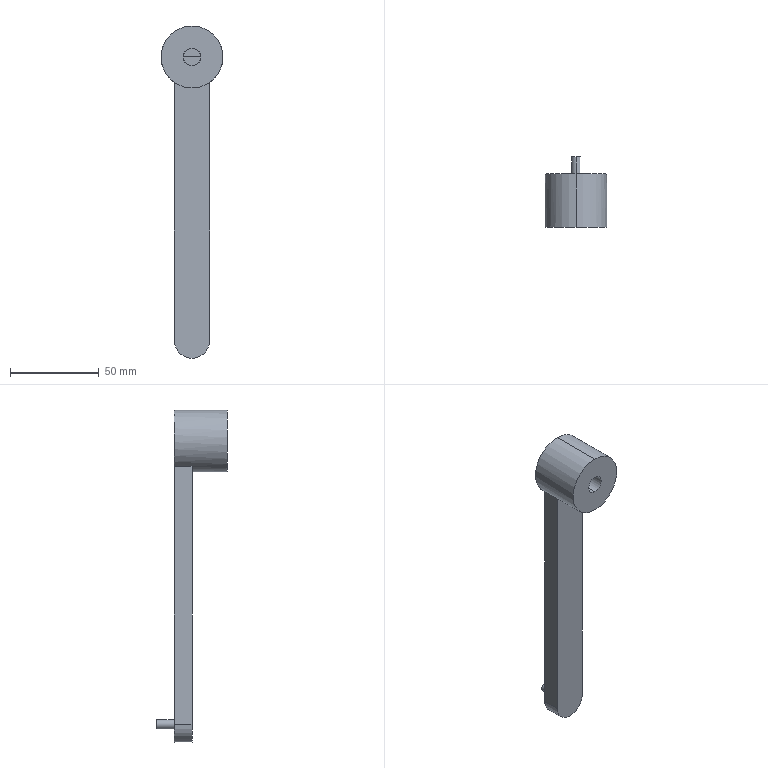Part | SolidWorks | features ICE 3, Extrusion 1 | 1 solid | 16 faces | box 35 x 40 x 187.5 mm | volume 57604 mm3 | plane 9 | cylinder 7 | commonest cylinder face diameters 5 x2 10 x2 35 x2 20 x1
STEP:
#1=CARTESIAN_POINT('',(0.,40.,-157.5));
#2=VERTEX_POINT('',#1);
#3=CARTESIAN_POINT('',(0.,40.,-162.5));
#4=VERTEX_POINT('',#3);
#5=CARTESIAN_POINT('',(0.,40.,-160.));
#6=DIRECTION('',(0.,1.,0.));
#7=DIRECTION('',(0.,0.,1.));
#8=AXIS2_PLACEMENT_3D('',#5,#6,#7);
#9=CIRCLE('',#8,2.5);
#10=EDGE_CURVE('',#2,#4,#9,.T.);
#11=ORIENTED_EDGE('',*,*,#10,.F.);
#12=CARTESIAN_POINT('',(0.,30.,-157.5));
#13=VERTEX_POINT('',#12);
#14=CARTESIAN_POINT('',(0.,40.,-157.5));
#15=DIRECTION('',(0.,-1.,0.));
#16=VECTOR('',#15,1000.);
#17=LINE('',#14,#16);
#18=EDGE_CURVE('',#2,#13,#17,.T.);
#19=ORIENTED_EDGE('',*,*,#18,.T.);
#20=CARTESIAN_POINT('',(0.,30.,-162.5));
#21=VERTEX_POINT('',#20);
#22=CARTESIAN_POINT('',(0.,30.,-160.));
#23=DIRECTION('',(0.,1.,0.));
#24=DIRECTION('',(0.,0.,1.));
#25=AXIS2_PLACEMENT_3D('',#22,#23,#24);
#26=CIRCLE('',#25,2.5);
#27=EDGE_CURVE('',#13,#21,#26,.T.);
#28=ORIENTED_EDGE('',*,*,#27,.T.);
#29=CARTESIAN_POINT('',(0.,40.,-162.5));
#30=DIRECTION('',(0.,-1.,0.));
#31=VECTOR('',#30,1000.);
#32=LINE('',#29,#31);
#33=EDGE_CURVE('',#4,#21,#32,.T.);
#34=ORIENTED_EDGE('',*,*,#33,.F.);
#35=EDGE_LOOP('',(#11,#19,#28,#34));
#36=FACE_OUTER_BOUND('',#35,.T.);
#37=CARTESIAN_POINT('',(0.,40.,-160.));
#38=DIRECTION('',(0.,-1.,0.));
#39=DIRECTION('',(0.,0.,-1.));
#40=AXIS2_PLACEMENT_3D('',#37,#38,#39);
#41=CYLINDRICAL_SURFACE('',#40,2.5);
#42=ADVANCED_FACE('',(#36),#41,.T.);
#43=CARTESIAN_POINT('',(0.,24.,5.));
#44=VERTEX_POINT('',#43);
#45=CARTESIAN_POINT('',(-5.,24.,0.));
#46=VERTEX_POINT('',#45);
#47=CARTESIAN_POINT('',(0.,24.,0.));
#48=DIRECTION('',(0.,-1.,0.));
#49=DIRECTION('',(0.,0.,-1.));
#50=AXIS2_PLACEMENT_3D('',#47,#48,#49);
#51=CIRCLE('',#50,5.);
#52=EDGE_CURVE('',#44,#46,#51,.T.);
#53=ORIENTED_EDGE('',*,*,#52,.F.);
#54=CARTESIAN_POINT('',(0.,0.,5.));
#55=VERTEX_POINT('',#54);
#56=CARTESIAN_POINT('',(0.,24.,5.));
#57=DIRECTION('',(0.,-1.,0.));
#58=VECTOR('',#57,1000.);
#59=LINE('',#56,#58);
#60=EDGE_CURVE('',#44,#55,#59,.T.);
#61=ORIENTED_EDGE('',*,*,#60,.T.);
#62=CARTESIAN_POINT('',(0.,0.,-5.));
#63=VERTEX_POINT('',#62);
#64=CARTESIAN_POINT('',(0.,0.,0.));
#65=DIRECTION('',(0.,-1.,0.));
#66=DIRECTION('',(0.,0.,-1.));
#67=AXIS2_PLACEMENT_3D('',#64,#65,#66);
#68=CIRCLE('',#67,5.);
#69=EDGE_CURVE('',#55,#63,#68,.T.);
#70=ORIENTED_EDGE('',*,*,#69,.T.);
#71=CARTESIAN_POINT('',(0.,20.,-5.));
#72=VERTEX_POINT('',#71);
#73=CARTESIAN_POINT('',(0.,24.,-5.));
#74=DIRECTION('',(0.,-1.,0.));
#75=VECTOR('',#74,1000.);
#76=LINE('',#73,#75);
#77=EDGE_CURVE('',#72,#63,#76,.T.);
#78=ORIENTED_EDGE('',*,*,#77,.F.);
#79=CARTESIAN_POINT('',(-5.,20.,0.));
#80=VERTEX_POINT('',#79);
#81=CARTESIAN_POINT('',(0.,20.,0.));
#82=DIRECTION('',(0.,-1.,0.));
#83=DIRECTION('',(0.,0.,1.));
#84=AXIS2_PLACEMENT_3D('',#81,#82,#83);
#85=CIRCLE('',#84,5.);
#86=EDGE_CURVE('',#80,#72,#85,.T.);
#87=ORIENTED_EDGE('',*,*,#86,.F.);
#88=CARTESIAN_POINT('',(-5.,24.,0.));
#89=DIRECTION('',(0.,1.,0.));
#90=VECTOR('',#89,1000.);
#91=LINE('',#88,#90);
#92=EDGE_CURVE('',#80,#46,#91,.T.);
#93=ORIENTED_EDGE('',*,*,#92,.T.);
#94=EDGE_LOOP('',(#53,#61,#70,#78,#87,#93));
#95=FACE_OUTER_BOUND('',#94,.T.);
#96=CARTESIAN_POINT('',(0.,24.,0.));
#97=DIRECTION('',(0.,-1.,0.));
#98=DIRECTION('',(0.,0.,-1.));
#99=AXIS2_PLACEMENT_3D('',#96,#97,#98);
#100=CYLINDRICAL_SURFACE('',#99,5.);
#101=ADVANCED_FACE('',(#95),#100,.F.);
#102=CARTESIAN_POINT('',(0.,30.,17.5));
#103=VERTEX_POINT('',#102);
#104=CARTESIAN_POINT('',(10.,30.,-14.361));
#105=VERTEX_POINT('',#104);
#106=CARTESIAN_POINT('',(0.,30.,0.));
#107=DIRECTION('',(0.,1.,0.));
#108=DIRECTION('',(0.,0.,1.));
#109=AXIS2_PLACEMENT_3D('',#106,#107,#108);
#110=CIRCLE('',#109,17.5);
#111=EDGE_CURVE('',#103,#105,#110,.T.);
#112=ORIENTED_EDGE('',*,*,#111,.F.);
#113=CARTESIAN_POINT('',(0.,0.,17.5));
#114=VERTEX_POINT('',#113);
#115=CARTESIAN_POINT('',(0.,30.,17.5));
#116=DIRECTION('',(0.,-1.,0.));
#117=VECTOR('',#116,1000.);
#118=LINE('',#115,#117);
#119=EDGE_CURVE('',#103,#114,#118,.T.);
#120=ORIENTED_EDGE('',*,*,#119,.T.);
#121=CARTESIAN_POINT('',(0.,0.,-17.5));
#122=VERTEX_POINT('',#121);
#123=CARTESIAN_POINT('',(0.,0.,0.));
#124=DIRECTION('',(0.,1.,0.));
#125=DIRECTION('',(0.,0.,1.));
#126=AXIS2_PLACEMENT_3D('',#123,#124,#125);
#127=CIRCLE('',#126,17.5);
#128=EDGE_CURVE('',#114,#122,#127,.T.);
#129=ORIENTED_EDGE('',*,*,#128,.T.);
#130=CARTESIAN_POINT('',(0.,20.,-17.5));
#131=VERTEX_POINT('',#130);
#132=CARTESIAN_POINT('',(0.,30.,-17.5));
#133=DIRECTION('',(0.,-1.,0.));
#134=VECTOR('',#133,1000.);
#135=LINE('',#132,#134);
#136=EDGE_CURVE('',#131,#122,#135,.T.);
#137=ORIENTED_EDGE('',*,*,#136,.F.);
#138=CARTESIAN_POINT('',(10.,20.,-14.361));
#139=VERTEX_POINT('',#138);
#140=CARTESIAN_POINT('',(0.,20.,0.));
#141=DIRECTION('',(0.,1.,0.));
#142=DIRECTION('',(0.,0.,1.));
#143=AXIS2_PLACEMENT_3D('',#140,#141,#142);
#144=CIRCLE('',#143,17.5);
#145=EDGE_CURVE('',#139,#131,#144,.T.);
#146=ORIENTED_EDGE('',*,*,#145,.F.);
#147=CARTESIAN_POINT('',(10.,30.,-14.361));
#148=DIRECTION('',(0.,1.,0.));
#149=VECTOR('',#148,1000.);
#150=LINE('',#147,#149);
#151=EDGE_CURVE('',#139,#105,#150,.T.);
#152=ORIENTED_EDGE('',*,*,#151,.T.);
#153=EDGE_LOOP('',(#112,#120,#129,#137,#146,#152));
#154=FACE_OUTER_BOUND('',#153,.T.);
#155=CARTESIAN_POINT('',(0.,30.,0.));
#156=DIRECTION('',(0.,-1.,0.));
#157=DIRECTION('',(0.,0.,-1.));
#158=AXIS2_PLACEMENT_3D('',#155,#156,#157);
#159=CYLINDRICAL_SURFACE('',#158,17.5);
#160=ADVANCED_FACE('',(#154),#159,.T.);
#161=CARTESIAN_POINT('',(-10.,30.,-14.361));
#162=VERTEX_POINT('',#161);
#163=CARTESIAN_POINT('',(0.,30.,0.));
#164=DIRECTION('',(0.,1.,0.));
#165=DIRECTION('',(0.,0.,1.));
#166=AXIS2_PLACEMENT_3D('',#163,#164,#165);
#167=CIRCLE('',#166,17.5);
#168=EDGE_CURVE('',#162,#103,#167,.T.);
#169=ORIENTED_EDGE('',*,*,#168,.T.);
#170=ORIENTED_EDGE('',*,*,#111,.T.);
#171=CARTESIAN_POINT('',(10.,30.,-160.));
#172=VERTEX_POINT('',#171);
#173=CARTESIAN_POINT('',(10.,30.,-160.));
#174=DIRECTION('',(0.,0.,-1.));
#175=VECTOR('',#174,1000.);
#176=LINE('',#173,#175);
#177=EDGE_CURVE('',#105,#172,#176,.T.);
#178=ORIENTED_EDGE('',*,*,#177,.T.);
#179=CARTESIAN_POINT('',(-10.,30.,-160.));
#180=VERTEX_POINT('',#179);
#181=CARTESIAN_POINT('',(0.,30.,-160.));
#182=DIRECTION('',(0.,1.,0.));
#183=DIRECTION('',(0.,0.,1.));
#184=AXIS2_PLACEMENT_3D('',#181,#182,#183);
#185=CIRCLE('',#184,10.);
#186=EDGE_CURVE('',#172,#180,#185,.T.);
#187=ORIENTED_EDGE('',*,*,#186,.T.);
#188=CARTESIAN_POINT('',(-10.,30.,-160.));
#189=DIRECTION('',(0.,0.,1.));
#190=VECTOR('',#189,1000.);
#191=LINE('',#188,#190);
#192=EDGE_CURVE('',#180,#162,#191,.T.);
#193=ORIENTED_EDGE('',*,*,#192,.T.);
#194=EDGE_LOOP('',(#169,#170,#178,#187,#193));
#195=FACE_OUTER_BOUND('',#194,.T.);
#196=CARTESIAN_POINT('',(0.,30.,-160.));
#197=DIRECTION('',(0.,1.,0.));
#198=DIRECTION('',(0.,0.,1.));
#199=AXIS2_PLACEMENT_3D('',#196,#197,#198);
#200=CIRCLE('',#199,2.5);
#201=EDGE_CURVE('',#21,#13,#200,.T.);
#202=ORIENTED_EDGE('',*,*,#201,.F.);
#203=ORIENTED_EDGE('',*,*,#27,.F.);
#204=EDGE_LOOP('',(#202,#203));
#205=FACE_BOUND('',#204,.T.);
#206=CARTESIAN_POINT('',(0.,30.,0.));
#207=DIRECTION('',(0.,1.,0.));
#208=DIRECTION('',(0.,0.,1.));
#209=AXIS2_PLACEMENT_3D('',#206,#207,#208);
#210=PLANE('',#209);
#211=ADVANCED_FACE('',(#195,#205),#210,.T.);
#212=ORIENTED_EDGE('',*,*,#119,.F.);
#213=ORIENTED_EDGE('',*,*,#168,.F.);
#214=CARTESIAN_POINT('',(-10.,20.,-14.361));
#215=VERTEX_POINT('',#214);
#216=CARTESIAN_POINT('',(-10.,30.,-14.361));
#217=DIRECTION('',(0.,-1.,0.));
#218=VECTOR('',#217,1000.);
#219=LINE('',#216,#218);
#220=EDGE_CURVE('',#162,#215,#219,.T.);
#221=ORIENTED_EDGE('',*,*,#220,.T.);
#222=CARTESIAN_POINT('',(0.,20.,0.));
#223=DIRECTION('',(0.,1.,0.));
#224=DIRECTION('',(0.,0.,1.));
#225=AXIS2_PLACEMENT_3D('',#222,#223,#224);
#226=CIRCLE('',#225,17.5);
#227=EDGE_CURVE('',#131,#215,#226,.T.);
#228=ORIENTED_EDGE('',*,*,#227,.F.);
#229=ORIENTED_EDGE('',*,*,#136,.T.);
#230=CARTESIAN_POINT('',(0.,0.,0.));
#231=DIRECTION('',(0.,1.,0.));
#232=DIRECTION('',(0.,0.,1.));
#233=AXIS2_PLACEMENT_3D('',#230,#231,#232);
#234=CIRCLE('',#233,17.5);
#235=EDGE_CURVE('',#122,#114,#234,.T.);
#236=ORIENTED_EDGE('',*,*,#235,.T.);
#237=EDGE_LOOP('',(#212,#213,#221,#228,#229,#236));
#238=FACE_OUTER_BOUND('',#237,.T.);
#239=CARTESIAN_POINT('',(0.,30.,0.));
#240=DIRECTION('',(0.,-1.,0.));
#241=DIRECTION('',(0.,0.,-1.));
#242=AXIS2_PLACEMENT_3D('',#239,#240,#241);
#243=CYLINDRICAL_SURFACE('',#242,17.5);
#244=ADVANCED_FACE('',(#238),#243,.T.);
#245=CARTESIAN_POINT('',(0.,0.,0.));
#246=DIRECTION('',(0.,-1.,0.));
#247=DIRECTION('',(0.,0.,-1.));
#248=AXIS2_PLACEMENT_3D('',#245,#246,#247);
#249=CIRCLE('',#248,5.);
#250=EDGE_CURVE('',#63,#55,#249,.T.);
#251=ORIENTED_EDGE('',*,*,#250,.F.);
#252=ORIENTED_EDGE('',*,*,#69,.F.);
#253=EDGE_LOOP('',(#251,#252));
#254=FACE_BOUND('',#253,.T.);
#255=ORIENTED_EDGE('',*,*,#235,.F.);
#256=ORIENTED_EDGE('',*,*,#128,.F.);
#257=EDGE_LOOP('',(#255,#256));
#258=FACE_OUTER_BOUND('',#257,.T.);
#259=CARTESIAN_POINT('',(0.,0.,0.));
#260=DIRECTION('',(0.,1.,0.));
#261=DIRECTION('',(0.,0.,1.));
#262=AXIS2_PLACEMENT_3D('',#259,#260,#261);
#263=PLANE('',#262);
#264=ADVANCED_FACE('',(#254,#258),#263,.F.);
#265=ORIENTED_EDGE('',*,*,#60,.F.);
#266=CARTESIAN_POINT('',(5.,24.,0.));
#267=VERTEX_POINT('',#266);
#268=CARTESIAN_POINT('',(0.,24.,0.));
#269=DIRECTION('',(0.,-1.,0.));
#270=DIRECTION('',(0.,0.,-1.));
#271=AXIS2_PLACEMENT_3D('',#268,#269,#270);
#272=CIRCLE('',#271,5.);
#273=EDGE_CURVE('',#267,#44,#272,.T.);
#274=ORIENTED_EDGE('',*,*,#273,.F.);
#275=CARTESIAN_POINT('',(5.,20.,0.));
#276=VERTEX_POINT('',#275);
#277=CARTESIAN_POINT('',(5.,24.,0.));
#278=DIRECTION('',(0.,-1.,0.));
#279=VECTOR('',#278,1000.);
#280=LINE('',#277,#279);
#281=EDGE_CURVE('',#267,#276,#280,.T.);
#282=ORIENTED_EDGE('',*,*,#281,.T.);
#283=CARTESIAN_POINT('',(0.,20.,0.));
#284=DIRECTION('',(0.,-1.,0.));
#285=DIRECTION('',(0.,0.,1.));
#286=AXIS2_PLACEMENT_3D('',#283,#284,#285);
#287=CIRCLE('',#286,5.);
#288=EDGE_CURVE('',#72,#276,#287,.T.);
#289=ORIENTED_EDGE('',*,*,#288,.F.);
#290=ORIENTED_EDGE('',*,*,#77,.T.);
#291=ORIENTED_EDGE('',*,*,#250,.T.);
#292=EDGE_LOOP('',(#265,#274,#282,#289,#290,#291));
#293=FACE_OUTER_BOUND('',#292,.T.);
#294=CARTESIAN_POINT('',(0.,24.,0.));
#295=DIRECTION('',(0.,-1.,0.));
#296=DIRECTION('',(0.,0.,-1.));
#297=AXIS2_PLACEMENT_3D('',#294,#295,#296);
#298=CYLINDRICAL_SURFACE('',#297,5.);
#299=ADVANCED_FACE('',(#293),#298,.F.);
#300=CARTESIAN_POINT('',(0.,24.,0.));
#301=DIRECTION('',(-1.,0.,0.));
#302=VECTOR('',#301,1000.);
#303=LINE('',#300,#302);
#304=EDGE_CURVE('',#267,#46,#303,.T.);
#305=ORIENTED_EDGE('',*,*,#304,.F.);
#306=ORIENTED_EDGE('',*,*,#273,.T.);
#307=ORIENTED_EDGE('',*,*,#52,.T.);
#308=EDGE_LOOP('',(#305,#306,#307));
#309=FACE_OUTER_BOUND('',#308,.T.);
#310=CARTESIAN_POINT('',(0.,24.,0.));
#311=DIRECTION('',(0.,-1.,0.));
#312=DIRECTION('',(0.,0.,-1.));
#313=AXIS2_PLACEMENT_3D('',#310,#311,#312);
#314=PLANE('',#313);
#315=ADVANCED_FACE('',(#309),#314,.T.);
#316=ORIENTED_EDGE('',*,*,#92,.F.);
#317=CARTESIAN_POINT('',(-10.,20.,0.));
#318=DIRECTION('',(1.,0.,0.));
#319=VECTOR('',#318,1000.);
#320=LINE('',#317,#319);
#321=EDGE_CURVE('',#80,#276,#320,.T.);
#322=ORIENTED_EDGE('',*,*,#321,.T.);
#323=ORIENTED_EDGE('',*,*,#281,.F.);
#324=ORIENTED_EDGE('',*,*,#304,.T.);
#325=EDGE_LOOP('',(#316,#322,#323,#324));
#326=FACE_OUTER_BOUND('',#325,.T.);
#327=CARTESIAN_POINT('',(-10.,20.,0.));
#328=DIRECTION('',(0.,0.,1.));
#329=DIRECTION('',(1.,0.,0.));
#330=AXIS2_PLACEMENT_3D('',#327,#328,#329);
#331=PLANE('',#330);
#332=ADVANCED_FACE('',(#326),#331,.T.);
#333=ORIENTED_EDGE('',*,*,#321,.F.);
#334=ORIENTED_EDGE('',*,*,#86,.T.);
#335=ORIENTED_EDGE('',*,*,#288,.T.);
#336=EDGE_LOOP('',(#333,#334,#335));
#337=FACE_OUTER_BOUND('',#336,.T.);
#338=CARTESIAN_POINT('',(0.,20.,-160.));
#339=DIRECTION('',(0.,1.,0.));
#340=DIRECTION('',(0.,0.,1.));
#341=AXIS2_PLACEMENT_3D('',#338,#339,#340);
#342=PLANE('',#341);
#343=ADVANCED_FACE('',(#337),#342,.F.);
#344=ORIENTED_EDGE('',*,*,#151,.F.);
#345=CARTESIAN_POINT('',(10.,20.,-160.));
#346=VERTEX_POINT('',#345);
#347=CARTESIAN_POINT('',(10.,20.,-160.));
#348=DIRECTION('',(0.,0.,-1.));
#349=VECTOR('',#348,1000.);
#350=LINE('',#347,#349);
#351=EDGE_CURVE('',#139,#346,#350,.T.);
#352=ORIENTED_EDGE('',*,*,#351,.T.);
#353=CARTESIAN_POINT('',(10.,20.,-160.));
#354=DIRECTION('',(0.,1.,0.));
#355=VECTOR('',#354,1000.);
#356=LINE('',#353,#355);
#357=EDGE_CURVE('',#346,#172,#356,.T.);
#358=ORIENTED_EDGE('',*,*,#357,.T.);
#359=ORIENTED_EDGE('',*,*,#177,.F.);
#360=EDGE_LOOP('',(#344,#352,#358,#359));
#361=FACE_OUTER_BOUND('',#360,.T.);
#362=CARTESIAN_POINT('',(10.,20.,-160.));
#363=DIRECTION('',(1.,0.,0.));
#364=DIRECTION('',(0.,0.,-1.));
#365=AXIS2_PLACEMENT_3D('',#362,#363,#364);
#366=PLANE('',#365);
#367=ADVANCED_FACE('',(#361),#366,.T.);
#368=ORIENTED_EDGE('',*,*,#220,.F.);
#369=ORIENTED_EDGE('',*,*,#192,.F.);
#370=CARTESIAN_POINT('',(-10.,20.,-160.));
#371=VERTEX_POINT('',#370);
#372=CARTESIAN_POINT('',(-10.,20.,-160.));
#373=DIRECTION('',(0.,1.,0.));
#374=VECTOR('',#373,1000.);
#375=LINE('',#372,#374);
#376=EDGE_CURVE('',#371,#180,#375,.T.);
#377=ORIENTED_EDGE('',*,*,#376,.F.);
#378=CARTESIAN_POINT('',(-10.,20.,-160.));
#379=DIRECTION('',(0.,0.,1.));
#380=VECTOR('',#379,1000.);
#381=LINE('',#378,#380);
#382=EDGE_CURVE('',#371,#215,#381,.T.);
#383=ORIENTED_EDGE('',*,*,#382,.T.);
#384=EDGE_LOOP('',(#368,#369,#377,#383));
#385=FACE_OUTER_BOUND('',#384,.T.);
#386=CARTESIAN_POINT('',(-10.,20.,-160.));
#387=DIRECTION('',(-1.,0.,0.));
#388=DIRECTION('',(0.,0.,1.));
#389=AXIS2_PLACEMENT_3D('',#386,#387,#388);
#390=PLANE('',#389);
#391=ADVANCED_FACE('',(#385),#390,.T.);
#392=ORIENTED_EDGE('',*,*,#351,.F.);
#393=ORIENTED_EDGE('',*,*,#145,.T.);
#394=ORIENTED_EDGE('',*,*,#227,.T.);
#395=ORIENTED_EDGE('',*,*,#382,.F.);
#396=CARTESIAN_POINT('',(0.,20.,-160.));
#397=DIRECTION('',(0.,1.,0.));
#398=DIRECTION('',(0.,0.,1.));
#399=AXIS2_PLACEMENT_3D('',#396,#397,#398);
#400=CIRCLE('',#399,10.);
#401=EDGE_CURVE('',#346,#371,#400,.T.);
#402=ORIENTED_EDGE('',*,*,#401,.F.);
#403=EDGE_LOOP('',(#392,#393,#394,#395,#402));
#404=FACE_OUTER_BOUND('',#403,.T.);
#405=CARTESIAN_POINT('',(0.,20.,-160.));
#406=DIRECTION('',(0.,1.,0.));
#407=DIRECTION('',(0.,0.,1.));
#408=AXIS2_PLACEMENT_3D('',#405,#406,#407);
#409=PLANE('',#408);
#410=ADVANCED_FACE('',(#404),#409,.F.);
#411=ORIENTED_EDGE('',*,*,#186,.F.);
#412=ORIENTED_EDGE('',*,*,#357,.F.);
#413=ORIENTED_EDGE('',*,*,#401,.T.);
#414=ORIENTED_EDGE('',*,*,#376,.T.);
#415=EDGE_LOOP('',(#411,#412,#413,#414));
#416=FACE_OUTER_BOUND('',#415,.T.);
#417=CARTESIAN_POINT('',(0.,20.,-160.));
#418=DIRECTION('',(0.,1.,0.));
#419=DIRECTION('',(0.,0.,1.));
#420=AXIS2_PLACEMENT_3D('',#417,#418,#419);
#421=CYLINDRICAL_SURFACE('',#420,10.);
#422=ADVANCED_FACE('',(#416),#421,.T.);
#423=ORIENTED_EDGE('',*,*,#18,.F.);
#424=CARTESIAN_POINT('',(0.,40.,-160.));
#425=DIRECTION('',(0.,1.,0.));
#426=DIRECTION('',(0.,0.,1.));
#427=AXIS2_PLACEMENT_3D('',#424,#425,#426);
#428=CIRCLE('',#427,2.5);
#429=EDGE_CURVE('',#4,#2,#428,.T.);
#430=ORIENTED_EDGE('',*,*,#429,.F.);
#431=ORIENTED_EDGE('',*,*,#33,.T.);
#432=ORIENTED_EDGE('',*,*,#201,.T.);
#433=EDGE_LOOP('',(#423,#430,#431,#432));
#434=FACE_OUTER_BOUND('',#433,.T.);
#435=CARTESIAN_POINT('',(0.,40.,-160.));
#436=DIRECTION('',(0.,-1.,0.));
#437=DIRECTION('',(0.,0.,-1.));
#438=AXIS2_PLACEMENT_3D('',#435,#436,#437);
#439=CYLINDRICAL_SURFACE('',#438,2.5);
#440=ADVANCED_FACE('',(#434),#439,.T.);
#441=ORIENTED_EDGE('',*,*,#429,.T.);
#442=ORIENTED_EDGE('',*,*,#10,.T.);
#443=EDGE_LOOP('',(#441,#442));
#444=FACE_OUTER_BOUND('',#443,.T.);
#445=CARTESIAN_POINT('',(0.,40.,-160.));
#446=DIRECTION('',(0.,1.,0.));
#447=DIRECTION('',(0.,0.,1.));
#448=AXIS2_PLACEMENT_3D('',#445,#446,#447);
#449=PLANE('',#448);
#450=ADVANCED_FACE('',(#444),#449,.T.);
#451=CLOSED_SHELL('',(#42,#101,#160,#211,#244,#264,#299,#315,#332,#343,#367,#391,#410,#422,#440,#450));
#452=MANIFOLD_SOLID_BREP('',#451);
#453=CARTESIAN_POINT('',(0.,0.,0.));
#454=DIRECTION('',(0.,0.,1.));
#455=DIRECTION('',(1.,0.,0.));
#456=AXIS2_PLACEMENT_3D('',#453,#454,#455);
#457=(LENGTH_UNIT()NAMED_UNIT(*)SI_UNIT(.MILLI.,.METRE.));
#458=UNCERTAINTY_MEASURE_WITH_UNIT(LENGTH_MEASURE(0.00001),#457,'','');
#459=(NAMED_UNIT(*)PLANE_ANGLE_UNIT()SI_UNIT($,.RADIAN.));
#460=(NAMED_UNIT(*)SI_UNIT($,.STERADIAN.)SOLID_ANGLE_UNIT());
#461=(GEOMETRIC_REPRESENTATION_CONTEXT(3)GLOBAL_UNCERTAINTY_ASSIGNED_CONTEXT((#458))GLOBAL_UNIT_ASSIGNED_CONTEXT((#457,#459,#460))REPRESENTATION_CONTEXT('',''));
#462=ADVANCED_BREP_SHAPE_REPRESENTATION('',(#452,#456),#461);